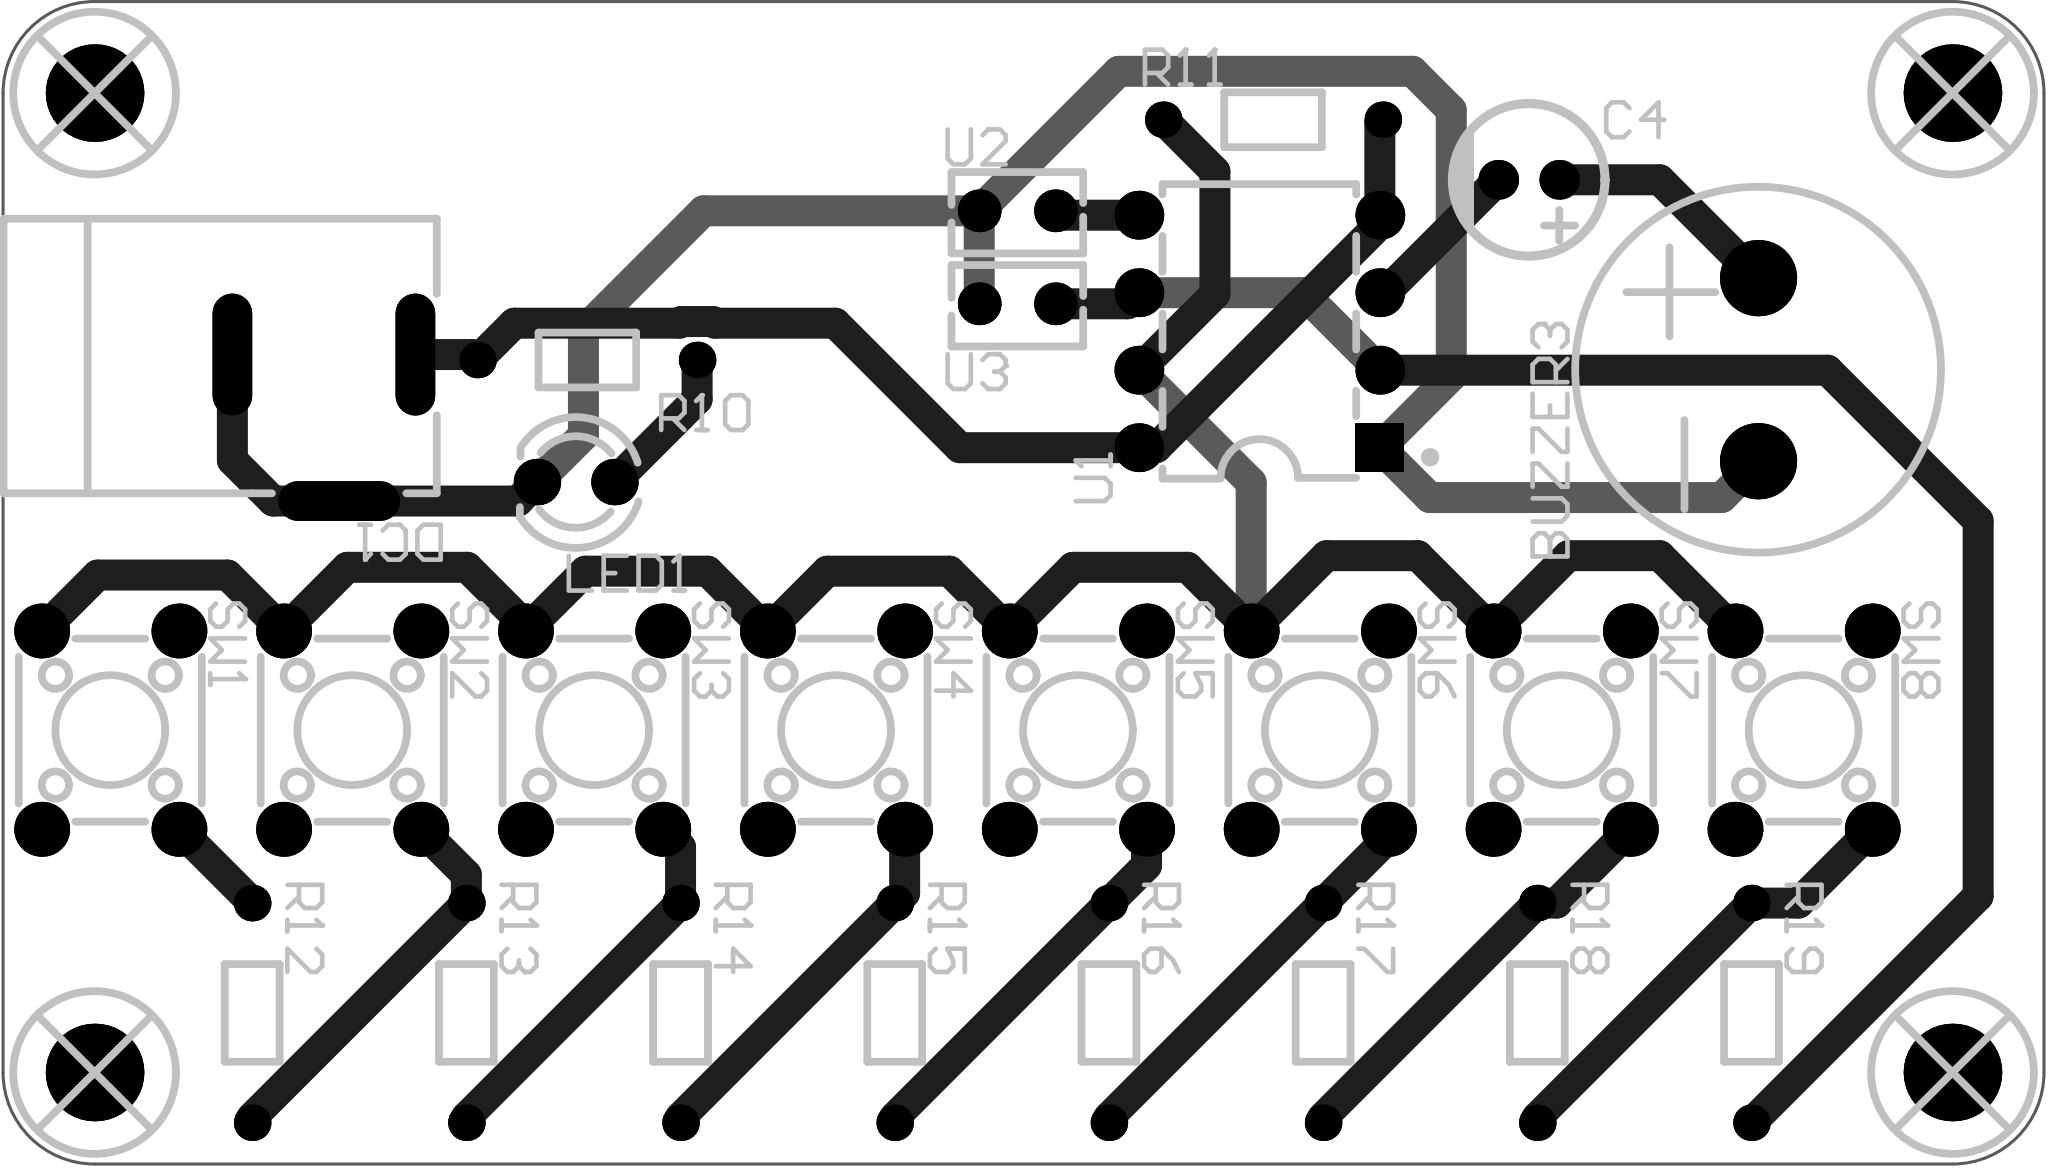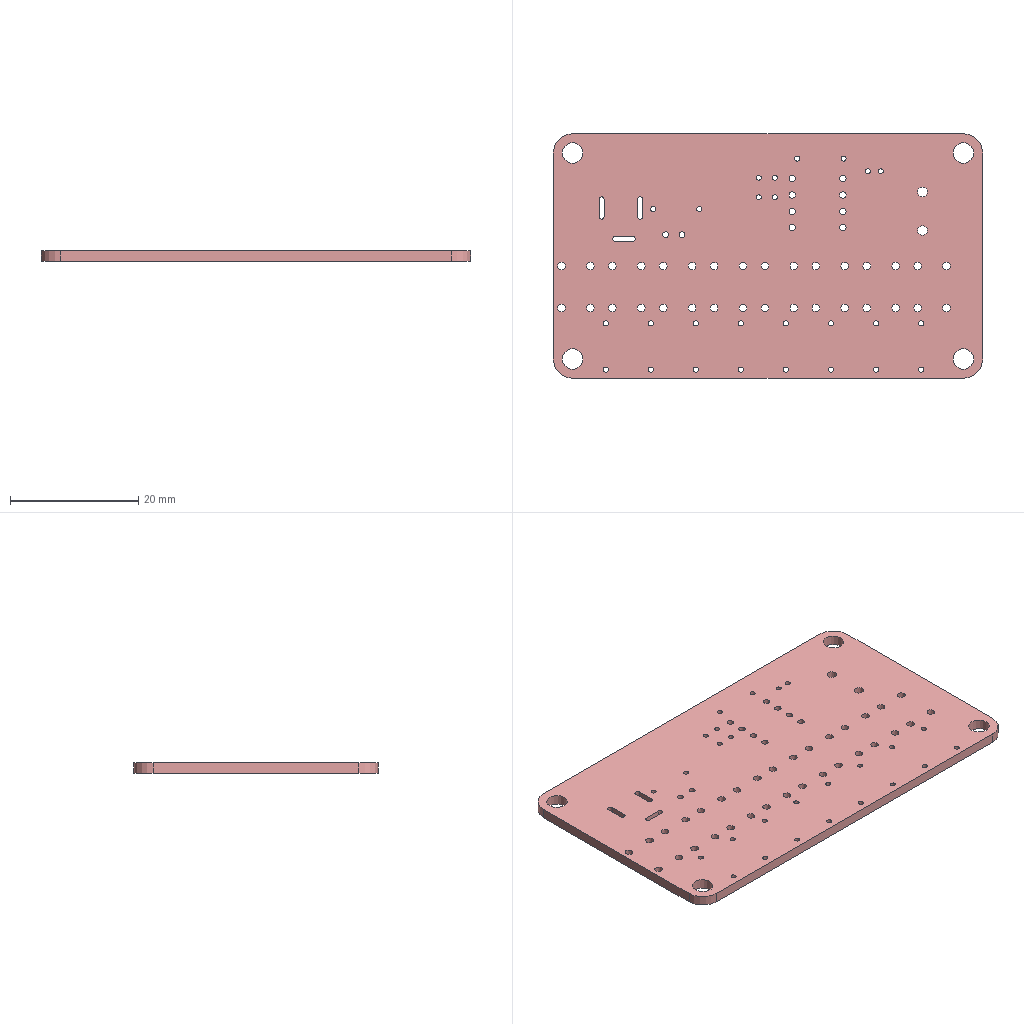Circuit board layout | Altium Designer | box 66.9 x 38.1 x 1.6 mm
Layer stack:
# Altium Designer layer stack of  (unit mm; dielectric type: 0 none, 1 core, 2 prepreg, 3 surface material)
index,name,kind,layer,copper_thickness_mm,dielectric_type,dielectric_thickness_mm,dielectric_material,dielectric_constant
0,Top Paste Mask Layer,other,,,,,,
1,Top Silkscreen Layer,other,,,,,,
2,Top Solder Mask Layer,dielectric,,,3,0.01,,3.3
3,Top Layer,copper,Top Layer,0.035,,,,
4,Dielectric1,dielectric,,,3,1.51,FR4,4.5
5,Bottom Layer,copper,Bottom Layer,0.035,,,,
6,Bottom Solder Mask Layer,dielectric,,,3,0.01,,3.3
7,Bottom Silkscreen Layer,other,,,,,,
8,Bottom Paste Mask Layer,other,,,,,,
# drill layer pairs: low layer,high layer
drill_pair,Top Layer,Bottom Layer
Part placement:
Designator,Comment,Layer,Footprint,Center-X(mm),Center-Y(mm),Rotation
C4,4.7uF,TopLayer,CAP-TH_BD5.0-P2.00-D0.8-FD,126.238,108.458,180
SCREW1,,TopLayer,M3螺丝,79.225,79.2,0
SCREW2,,TopLayer,M3螺丝,140.129,79.2,0
SCREW3,,TopLayer,M3螺丝,79.225,111.3,0
SCREW4,,TopLayer,M3螺丝,140.129,111.3,0
SW1,,TopLayer,SW-TH_4P-L6.0-W6.0-P4.50-LS6.5,79.74,90.421,270
SW2,,TopLayer,SW-TH_4P-L6.0-W6.0-P4.50-LS6.5,87.67,90.421,270
SW3,,TopLayer,SW-TH_4P-L6.0-W6.0-P4.50-LS6.5,95.6,90.421,270
SW4,,TopLayer,SW-TH_4P-L6.0-W6.0-P4.50-LS6.5,103.53,90.421,270
SW5,,TopLayer,SW-TH_4P-L6.0-W6.0-P4.50-LS6.5,111.46,90.421,270
SW6,,TopLayer,SW-TH_4P-L6.0-W6.0-P4.50-LS6.5,119.39,90.421,270
SW7,,TopLayer,SW-TH_4P-L6.0-W6.0-P4.50-LS6.5,127.32,90.421,270
SW8,,TopLayer,SW-TH_4P-L6.0-W6.0-P4.50-LS6.5,135.25,90.421,270
U1,NE555,TopLayer,PDIP-8_L9.6-W6.4-P2.54-LS7.9-BL-1,117.407,103.488,90
LED1,,TopLayer,LED_TH-3mm,94.996,98.552,180
R10,1kΩ,TopLayer,Res_1/8W,95.377,102.553,180
R11,1kΩ,TopLayer,Res_1/8W,117.856,110.426,0
R12,2kΩ,TopLayer,Res_1/8W,84.391,81.153,270
R13,2kΩ,TopLayer,Res_1/8W,91.412,81.153,270
R14,2kΩ,TopLayer,Res_1/8W,98.433,81.153,270
BUZZER3,buzzer,TopLayer,BUZ-TH_BD12.0-P6.00-D0.9-RD,133.756,102.235,90
R15,2kΩ,TopLayer,Res_1/8W,105.455,81.153,270
R16,2kΩ,TopLayer,Res_1/8W,112.476,81.153,270
R17,2kΩ,TopLayer,Res_1/8W,119.497,81.153,270
R18,2kΩ,TopLayer,Res_1/8W,126.519,81.153,270
R19,2kΩ,TopLayer,Res_1/8W,133.54,81.153,270
U2,10nF,TopLayer,CAP-TH_L4.0-W2.5-P2.50-D0.5,109.474,107.442,0
U3,100nF,TopLayer,CAP-TH_L4.0-W2.5-P2.50-D0.5,109.474,104.394,0
DC1,,TopLayer,DC-2.0,86.741,100.33,180
Pad and via stacks:
# Altium Designer via and pad stacks of  (unit mm). Each distinct definition once, with the count of objects using it.
# via: kind,start_layer,end_layer,hole_mm,diameter_mm,mode(0 simple;1 top-mid-bottom;2 full stack),diameter_per_layer,count,example_net
# pad: kind,layer,hole_mm,hole_type(0 round;1 square;2 slot),plating,top_size,top_shape(1 round;2 rect;3 octagon;9 rounded rect),mid_size,bottom_size,mode,footprint,size_per_layer,count,example
pad,Multi-Layer,0.8,0,plated,1.3x1.3,1,1.3x1.3,1.3x1.3,0,CAP-TH_BD5.0-P2.00-D0.8-FD,,2,C4.1
pad,Multi-Layer,3.2,0,plated,3.2x3.2,1,3.2x3.2,3.2x3.2,0,M3\u00C2\u00DD\u00CB\u00BF,,4,SCREW1.1
pad,Multi-Layer,1.2,0,plated,1.8x1.8,1,1.8x1.8,1.8x1.8,0,SW-TH_4P-L6.0-W6.0-P4.50-LS6.5,,32,SW1.1
pad,Multi-Layer,1,0,plated,1.6x1.6,1,1.6x1.6,1.6x1.6,0,PDIP-8_L9.6-W6.4-P2.54-LS7.9-BL-1,,7,U1.8
pad,Multi-Layer,1,0,plated,1.6x1.6,2,1.6x1.6,1.6x1.6,0,PDIP-8_L9.6-W6.4-P2.54-LS7.9-BL-1,,1,U1.1
pad,Multi-Layer,0.9144,0,plated,1.524x1.524,1,1.524x1.524,1.524x1.524,0,LED_TH-3mm,,2,LED1.1
pad,Multi-Layer,0.8001,0,plated,1.199x1.199,1,1.199x1.199,1.199x1.199,0,Res_1/8W,,20,R10.1
pad,Multi-Layer,1.5,0,plated,2.5x2.5,1,2.5x2.5,2.5x2.5,0,BUZ-TH_BD12.0-P6.00-D0.9-RD,,2,BUZZER3.1
pad,Multi-Layer,0.8,0,plated,1.4x1.4,1,1.4x1.4,1.4x1.4,0,CAP-TH_L4.0-W2.5-P2.50-D0.5,,4,U2.2
pad,Multi-Layer,0.8001,2,plated,4x1.3,1,4x1.3,4x1.3,0,DC-2.0,,3,DC1.2